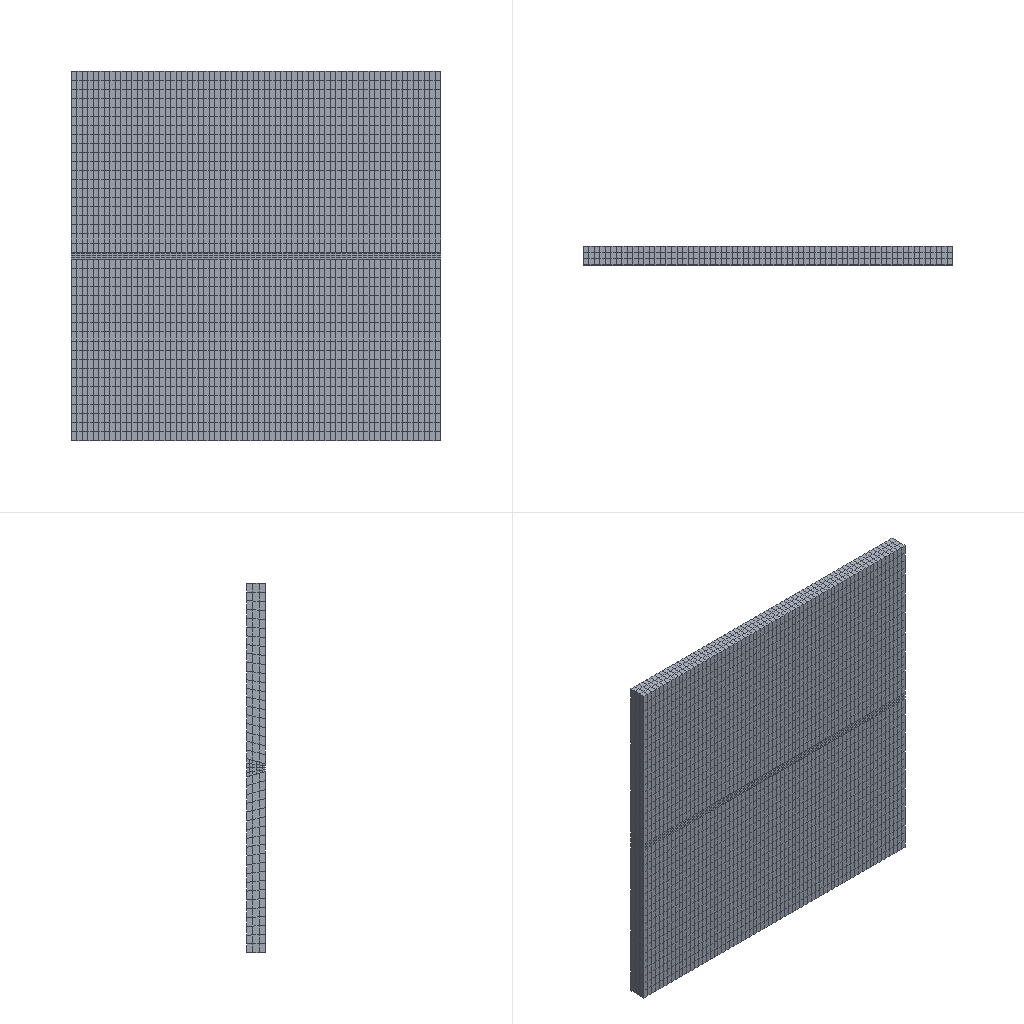Simulation study | abaqus
Set-up summary:
category,name,step,type,value,unit,region
solver,abaqus
solver,version,,,Abaqus/Standard 3DEXPERIENCE R2017x
units,not stated in the deck,,not stated
analysis,deck,,coupled temperature-displacement,coupled temperature-displacement
load_step,del-all,del-all,coupled temperature-displacement
load_step,add-1,add-1,coupled temperature-displacement
load_step,add-2,add-2,coupled temperature-displacement
load_step,requested,,,3
mesh,nodes,,,14959
mesh,elements,,,10440
element_type,C3D8RT,,solid,10440
load,load commands in deck,,count,1
bc,support commands in deck,,count,1
material,MATERIAL-1,,in results
check,setup vs results,,match,"per instance, exact: element labels, types and connectivity; labels of the nodes the elements use; coordinates of those nodes at SINGLE_PRECISION in 1 of 2 instance(s)"
Abaqus input file, long lists of numbers shortened:
*Heading
** Job name: Job-1 Model name: Model-1
** Generated by: Abaqus/CAE 2017
*Preprint, echo=NO, model=NO, history=NO, contact=NO
**
** PARTS
**
*Part, name=Part-1
*Node
      1,           0.,         -10.,   98.134
      2,           0.,           0.,   95.134
** (11422 more lines like these left out)
*Element, type=C3D8RT
   1,  232, 3297, 6409,  789,    1,   17,  713,   58
   2, 3297, 3298, 6410, 6409,   17,   18,  714,  713
** (8038 more lines like these left out)
*Nset, nset=Set-1, generate
     1,  11424,      1
*Elset, elset=Set-1, generate
    1,  8040,     1
** Section: Section-1
*Solid Section, elset=Set-1, material=Material-1
,
*End Part
**
*Part, name=han
*Node
      1,         200.,          -5.,   96.634
      2,         200.,          -5.,   103.634
** (3533 more lines like these left out)
*Element, type=C3D8RT
   1,  230, 1049, 2348,  653,    1,   13,  641,   22
   2, 1049, 1050, 2349, 2348,   13,   14,  642,  641
** (2398 more lines like these left out)
*Nset, nset=Set-1, generate
    1,  3535,     1
*Elset, elset=Set-1, generate
    1,  2400,     1
** Section: Section-1
*Solid Section, elset=Set-1, material=Material-1
,
*End Part
**
**
** ASSEMBLY
**
*Assembly, name=Assembly
**
*Instance, name=Part-1-1, part=Part-1
          0.,          10.,  -100.134
*End Instance
**
*Instance, name=han-1, part=han
          0.,          10.,  -100.134
*End Instance
**
*Nset, nset=Set-1, instance=han-1, generate
    1,  3535,     1
*Elset, elset=Set-1, instance=han-1, generate
    1,  2400,     1
*Nset, nset=Set-2, instance=han-1
    1,    2,    3,    4,    5,    6,    7,    8,   13,   14,   15,   16,   17,   18,   19,   20
   21,   22,   23,   24,   25,   26,   27,   28,   29,   30,   31,   32,   33,   34,   35,   36
** (125 more lines like these left out)
*Elset, elset=Set-2, instance=han-1, generate
    1,  1200,     1
*Nset, nset=Set-3, instance=han-1
    1,    2,    5,    8,    9,   10,   11,   12,   13,   14,   15,   23,   24,   25,  132,  133
  134,  135,  136,  137,  138,  139,  140,  141,  142,  143,  144,  145,  146,  147,  148,  149
** (125 more lines like these left out)
*Elset, elset=Set-3, instance=han-1, generate
 1201,  2400,     1
*Nset, nset=Set-4, instance=Part-1-1
    3,    4,    6,    7,   11,   12,   14,   15,   38,   39,   80,   81,  101,  102,  103,  104
  105,  106,  107,  108,  109,  110,  111,  112,  113,  114,  115,  116,  117,  118,  119,  120
** (32 more lines like these left out)
*Elset, elset=Set-4, instance=Part-1-1
   58,   59,   60,  118,  119,  120,  178,  179,  180,  238,  239,  240,  298,  299,  300,  358
  359,  360,  418,  419,  420,  478,  479,  480,  538,  539,  540,  598,  599,  600,  658,  659
** (24 more lines like these left out)
*Nset, nset=Set-5, instance=Part-1-1, generate
     1,  11424,      1
*Nset, nset=Set-5, instance=han-1, generate
    1,  3535,     1
*Elset, elset=Set-5, instance=Part-1-1, generate
    1,  8040,     1
*Elset, elset=Set-5, instance=han-1, generate
    1,  2400,     1
*Nset, nset=Set-6, instance=han-1, generate
    1,  3535,     1
*Elset, elset=Set-6, instance=han-1, generate
    1,  2400,     1
*Elset, elset=_m_Surf-1_S3, internal, instance=Part-1-1
    1,    2,    3,   61,   62,   63,  121,  122,  123,  181,  182,  183,  241,  242,  243,  301
  302,  303,  361,  362,  363,  421,  422,  423,  481,  482,  483,  541,  542,  543,  601,  602
** (24 more lines like these left out)
*Surface, type=ELEMENT, name=m_Surf-1
_m_Surf-1_S3, S3
*Elset, elset=_s_Surf-1_S4, internal, instance=han-1, generate
    4,  2400,     4
*Elset, elset=_s_Surf-1_S6, internal, instance=han-1, generate
    1,  2397,     4
*Surface, type=ELEMENT, name=s_Surf-1
_s_Surf-1_S4, S4
_s_Surf-1_S6, S6
** Constraint: Constraint-1
*Tie, name=Constraint-1, adjust=yes
s_Surf-1, m_Surf-1
*End Assembly
**
** MATERIALS
**
*Material, name=Material-1
*Conductivity
55.,
*Density
 7.8e-09,
*Elastic
210000., 0.3
*Expansion
 1.5e-05,
*Plastic
355.,0.
*Specific Heat
 4.6e+08,
**
** PREDEFINED FIELDS
**
** Name: Predefined Field-1   Type: Temperature
*Initial Conditions, type=TEMPERATURE
Set-5, 20.
** ----------------------------------------------------------------
**
** STEP: del-all
**
*Step, name=del-all, nlgeom=YES
*Coupled Temperature-displacement, creep=none, deltmx=1e+07, stabilize=0.0002, allsdtol=0.05, continue=NO
0.001, 0.001, 1e-08, 0.001
**
** BOUNDARY CONDITIONS
**
** Name: BC-1 Type: 对称/反对称/完全固定
*Boundary
Set-4, ENCASTRE
**
** INTERACTIONS
**
** Interaction: Int-del
*Model Change, remove
Set-1,
**
** OUTPUT REQUESTS
**
*Restart, write, frequency=0
**
** FIELD OUTPUT: F-Output-1
**
*Output, field
*Node Output
CF, NT, RF, RFL, RM, RT, TF, U
V
*Element Output, directions=YES
E, HFL, LE, MISES, MISESMAX, MISESONLY, PE, PEEQ, PEEQMAX, PEEQT, PEMAG, PRESSONLY, S, SF, SSAVG, TEMP
VEEQ
*Contact Output
CDISP, CSTRESS
*Radiation Output
FTEMP,
**
** HISTORY OUTPUT: H-Output-1
**
*Output, history, variable=PRESELECT
*End Step
** ----------------------------------------------------------------
**
** STEP: add-1
**
*Step, name=add-1, nlgeom=YES, inc=10000
*Coupled Temperature-displacement, creep=none, deltmx=1e+06, stabilize=0.0002, allsdtol=0.05, continue=NO
0.02, 4., 0.0001, 0.5
**
** LOADS
**
** Name: Load-1   Type: Body heat flux
*Dflux
Set-6, BFNU, 1.
**
** INTERACTIONS
**
** Interaction: Int-add1
*Model Change, add
Set-2,
**
** OUTPUT REQUESTS
**
*Restart, write, frequency=0
**
** FIELD OUTPUT: F-Output-1
**
*Output, field
*Node Output
CF, NT, RF, RFL, RM, RT, TF, U
V
*Element Output, directions=YES
E, HFL, LE, MISES, MISESMAX, MISESONLY, PE, PEEQ, PEEQMAX, PEEQT, PEMAG, PRESSONLY, S, SF, SSAVG, TEMP
VEEQ
*Contact Output
CDISP, CSTRESS
*Radiation Output
FTEMP,
**
** HISTORY OUTPUT: H-Output-1
**
*Output, history, variable=PRESELECT
*End Step
** ----------------------------------------------------------------
**
** STEP: add-2
**
*Step, name=add-2, nlgeom=YES, inc=10000
*Coupled Temperature-displacement, creep=none, deltmx=1e+07, stabilize=0.0002, allsdtol=0.05, continue=NO
0.02, 4., 0.0001, 0.1
**
** INTERACTIONS
**
** Interaction: Int-add2
*Model Change, add
Set-3,
**
** OUTPUT REQUESTS
**
*Restart, write, frequency=0
**
** FIELD OUTPUT: F-Output-1
**
*Output, field
*Node Output
CF, NT, RF, RFL, RM, RT, TF, U
V
*Element Output, directions=YES
E, HFL, LE, MISES, MISESMAX, MISESONLY, PE, PEEQ, PEEQMAX, PEEQT, PEMAG, PRESSONLY, S, SF, SSAVG, TEMP
VEEQ
*Contact Output
CDISP, CSTRESS
*Radiation Output
FTEMP,
**
** HISTORY OUTPUT: H-Output-1
**
*Output, history, variable=PRESELECT
*End Step
Results summary:
result,step,,completed,increments=1 time=0.001/0.001
result,step,,completed,increments=223 time=4.0/4.0
result,step,,completed,increments=53 time=4.0/4.0
result,analysis,,,"coupled temperature-displacement, steady state"
result,last_loadstep,,,3
result,primary field,,,"U, NT11"
result,reaction total,,FX,0.006014,model units
result,reaction total,,FY,0.9853,model units
result,reaction total,,FZ,0.000383,model units